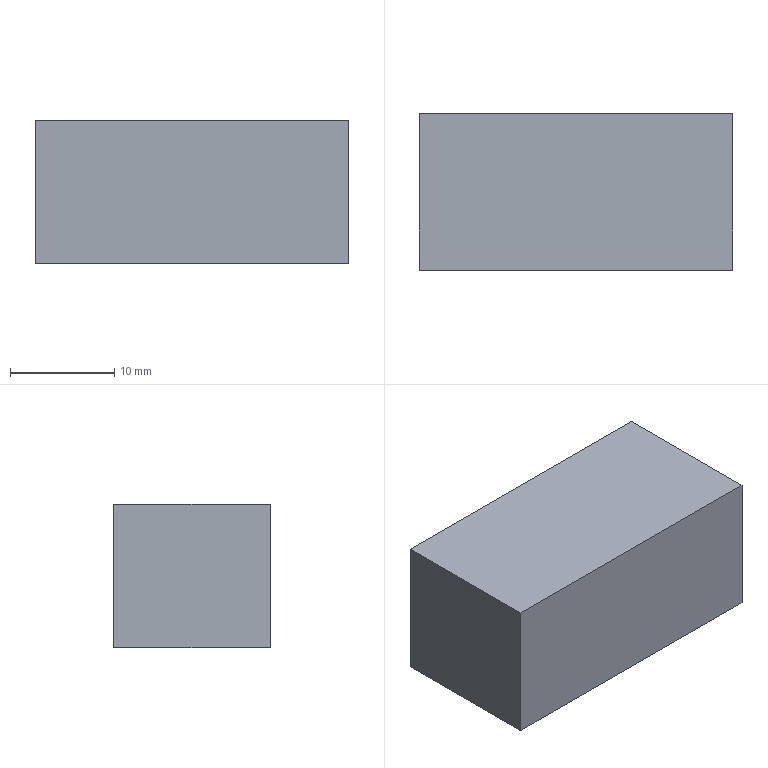Part | STEP file | 1105WW撞块-002_デフォルト | 1 solid | 6 faces | box 30 x 15 x 13.8 mm | volume 6210 mm3 | plane 6
STEP:
#1=CARTESIAN_POINT('',(15.,-7.5,0.));
#2=VERTEX_POINT('',#1);
#3=CARTESIAN_POINT('',(15.,7.5,0.));
#4=VERTEX_POINT('',#3);
#5=CARTESIAN_POINT('',(15.,7.5,0.));
#6=DIRECTION('',(0.,1.,0.));
#7=VECTOR('',#6,1000.);
#8=LINE('',#5,#7);
#9=EDGE_CURVE('',#2,#4,#8,.T.);
#10=ORIENTED_EDGE('',*,*,#9,.T.);
#11=CARTESIAN_POINT('',(15.,7.5,13.8));
#12=VERTEX_POINT('',#11);
#13=CARTESIAN_POINT('',(15.,7.5,13.8));
#14=DIRECTION('',(0.,0.,-1.));
#15=VECTOR('',#14,1000.);
#16=LINE('',#13,#15);
#17=EDGE_CURVE('',#12,#4,#16,.T.);
#18=ORIENTED_EDGE('',*,*,#17,.F.);
#19=CARTESIAN_POINT('',(15.,-7.5,13.8));
#20=VERTEX_POINT('',#19);
#21=CARTESIAN_POINT('',(15.,7.5,13.8));
#22=DIRECTION('',(0.,1.,0.));
#23=VECTOR('',#22,1000.);
#24=LINE('',#21,#23);
#25=EDGE_CURVE('',#20,#12,#24,.T.);
#26=ORIENTED_EDGE('',*,*,#25,.F.);
#27=CARTESIAN_POINT('',(15.,-7.5,13.8));
#28=DIRECTION('',(0.,0.,-1.));
#29=VECTOR('',#28,1000.);
#30=LINE('',#27,#29);
#31=EDGE_CURVE('',#20,#2,#30,.T.);
#32=ORIENTED_EDGE('',*,*,#31,.T.);
#33=EDGE_LOOP('',(#10,#18,#26,#32));
#34=FACE_OUTER_BOUND('',#33,.T.);
#35=CARTESIAN_POINT('',(15.,7.5,13.8));
#36=DIRECTION('',(-1.,0.,0.));
#37=DIRECTION('',(0.,-1.,0.));
#38=AXIS2_PLACEMENT_3D('',#35,#36,#37);
#39=PLANE('',#38);
#40=ADVANCED_FACE('',(#34),#39,.F.);
#41=CARTESIAN_POINT('',(-15.,7.5,0.));
#42=VERTEX_POINT('',#41);
#43=CARTESIAN_POINT('',(-15.,7.5,0.));
#44=DIRECTION('',(-1.,0.,0.));
#45=VECTOR('',#44,1000.);
#46=LINE('',#43,#45);
#47=EDGE_CURVE('',#4,#42,#46,.T.);
#48=ORIENTED_EDGE('',*,*,#47,.T.);
#49=CARTESIAN_POINT('',(-15.,7.5,13.8));
#50=VERTEX_POINT('',#49);
#51=CARTESIAN_POINT('',(-15.,7.5,13.8));
#52=DIRECTION('',(0.,0.,-1.));
#53=VECTOR('',#52,1000.);
#54=LINE('',#51,#53);
#55=EDGE_CURVE('',#50,#42,#54,.T.);
#56=ORIENTED_EDGE('',*,*,#55,.F.);
#57=CARTESIAN_POINT('',(-15.,7.5,13.8));
#58=DIRECTION('',(-1.,0.,0.));
#59=VECTOR('',#58,1000.);
#60=LINE('',#57,#59);
#61=EDGE_CURVE('',#12,#50,#60,.T.);
#62=ORIENTED_EDGE('',*,*,#61,.F.);
#63=ORIENTED_EDGE('',*,*,#17,.T.);
#64=EDGE_LOOP('',(#48,#56,#62,#63));
#65=FACE_OUTER_BOUND('',#64,.T.);
#66=CARTESIAN_POINT('',(-15.,7.5,13.8));
#67=DIRECTION('',(0.,-1.,0.));
#68=DIRECTION('',(0.,0.,-1.));
#69=AXIS2_PLACEMENT_3D('',#66,#67,#68);
#70=PLANE('',#69);
#71=ADVANCED_FACE('',(#65),#70,.F.);
#72=CARTESIAN_POINT('',(-15.,-7.5,0.));
#73=VERTEX_POINT('',#72);
#74=CARTESIAN_POINT('',(-15.,7.5,0.));
#75=DIRECTION('',(0.,-1.,0.));
#76=VECTOR('',#75,1000.);
#77=LINE('',#74,#76);
#78=EDGE_CURVE('',#42,#73,#77,.T.);
#79=ORIENTED_EDGE('',*,*,#78,.T.);
#80=CARTESIAN_POINT('',(-15.,-7.5,13.8));
#81=VERTEX_POINT('',#80);
#82=CARTESIAN_POINT('',(-15.,-7.5,13.8));
#83=DIRECTION('',(0.,0.,-1.));
#84=VECTOR('',#83,1000.);
#85=LINE('',#82,#84);
#86=EDGE_CURVE('',#81,#73,#85,.T.);
#87=ORIENTED_EDGE('',*,*,#86,.F.);
#88=CARTESIAN_POINT('',(-15.,7.5,13.8));
#89=DIRECTION('',(0.,-1.,0.));
#90=VECTOR('',#89,1000.);
#91=LINE('',#88,#90);
#92=EDGE_CURVE('',#50,#81,#91,.T.);
#93=ORIENTED_EDGE('',*,*,#92,.F.);
#94=ORIENTED_EDGE('',*,*,#55,.T.);
#95=EDGE_LOOP('',(#79,#87,#93,#94));
#96=FACE_OUTER_BOUND('',#95,.T.);
#97=CARTESIAN_POINT('',(-15.,7.5,13.8));
#98=DIRECTION('',(1.,0.,0.));
#99=DIRECTION('',(0.,1.,0.));
#100=AXIS2_PLACEMENT_3D('',#97,#98,#99);
#101=PLANE('',#100);
#102=ADVANCED_FACE('',(#96),#101,.F.);
#103=CARTESIAN_POINT('',(-15.,-7.5,0.));
#104=DIRECTION('',(1.,0.,0.));
#105=VECTOR('',#104,1000.);
#106=LINE('',#103,#105);
#107=EDGE_CURVE('',#73,#2,#106,.T.);
#108=ORIENTED_EDGE('',*,*,#107,.T.);
#109=ORIENTED_EDGE('',*,*,#31,.F.);
#110=CARTESIAN_POINT('',(-15.,-7.5,13.8));
#111=DIRECTION('',(1.,0.,0.));
#112=VECTOR('',#111,1000.);
#113=LINE('',#110,#112);
#114=EDGE_CURVE('',#81,#20,#113,.T.);
#115=ORIENTED_EDGE('',*,*,#114,.F.);
#116=ORIENTED_EDGE('',*,*,#86,.T.);
#117=EDGE_LOOP('',(#108,#109,#115,#116));
#118=FACE_OUTER_BOUND('',#117,.T.);
#119=CARTESIAN_POINT('',(-15.,-7.5,13.8));
#120=DIRECTION('',(0.,1.,0.));
#121=DIRECTION('',(0.,0.,1.));
#122=AXIS2_PLACEMENT_3D('',#119,#120,#121);
#123=PLANE('',#122);
#124=ADVANCED_FACE('',(#118),#123,.F.);
#125=ORIENTED_EDGE('',*,*,#25,.T.);
#126=ORIENTED_EDGE('',*,*,#61,.T.);
#127=ORIENTED_EDGE('',*,*,#92,.T.);
#128=ORIENTED_EDGE('',*,*,#114,.T.);
#129=EDGE_LOOP('',(#125,#126,#127,#128));
#130=FACE_OUTER_BOUND('',#129,.T.);
#131=CARTESIAN_POINT('',(0.,0.,13.8));
#132=DIRECTION('',(0.,0.,1.));
#133=DIRECTION('',(1.,0.,0.));
#134=AXIS2_PLACEMENT_3D('',#131,#132,#133);
#135=PLANE('',#134);
#136=ADVANCED_FACE('',(#130),#135,.T.);
#137=ORIENTED_EDGE('',*,*,#9,.F.);
#138=ORIENTED_EDGE('',*,*,#107,.F.);
#139=ORIENTED_EDGE('',*,*,#78,.F.);
#140=ORIENTED_EDGE('',*,*,#47,.F.);
#141=EDGE_LOOP('',(#137,#138,#139,#140));
#142=FACE_OUTER_BOUND('',#141,.T.);
#143=CARTESIAN_POINT('',(0.,0.,0.));
#144=DIRECTION('',(0.,0.,1.));
#145=DIRECTION('',(1.,0.,0.));
#146=AXIS2_PLACEMENT_3D('',#143,#144,#145);
#147=PLANE('',#146);
#148=ADVANCED_FACE('',(#142),#147,.F.);
#149=CLOSED_SHELL('',(#40,#71,#102,#124,#136,#148));
#150=MANIFOLD_SOLID_BREP('',#149);
#151=CARTESIAN_POINT('',(0.,0.,0.));
#152=DIRECTION('',(0.,0.,1.));
#153=DIRECTION('',(1.,0.,0.));
#154=AXIS2_PLACEMENT_3D('',#151,#152,#153);
#155=(LENGTH_UNIT()NAMED_UNIT(*)SI_UNIT(.MILLI.,.METRE.));
#156=UNCERTAINTY_MEASURE_WITH_UNIT(LENGTH_MEASURE(0.00001),#155,'','');
#157=(NAMED_UNIT(*)PLANE_ANGLE_UNIT()SI_UNIT($,.RADIAN.));
#158=(NAMED_UNIT(*)SI_UNIT($,.STERADIAN.)SOLID_ANGLE_UNIT());
#159=(GEOMETRIC_REPRESENTATION_CONTEXT(3)GLOBAL_UNCERTAINTY_ASSIGNED_CONTEXT((#156))GLOBAL_UNIT_ASSIGNED_CONTEXT((#155,#157,#158))REPRESENTATION_CONTEXT('',''));
#160=ADVANCED_BREP_SHAPE_REPRESENTATION('',(#150,#154),#159);